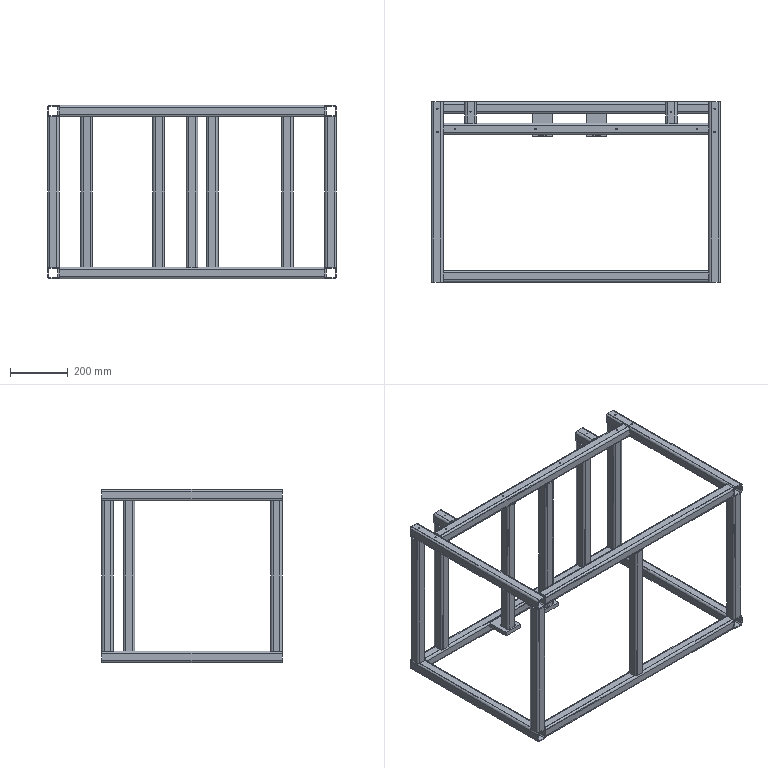Part | SolidWorks | features DelFace 22, WeldCornerFeat 15, CombineBodies 7, WeldMemberFeat 6, 3DProfileFeature 2, Boss 2, DeleteBody 2, HoleWzd 2, MoveCopyBody 2, WeldmentFeature 1 | 21 solids | 374 faces | box 1000 x 625 x 600 mm | volume 6055462 mm3 | plane 202 | cylinder 172 | commonest cylinder face diameters 8 x76 16 x76 4.2 x12 5 x8